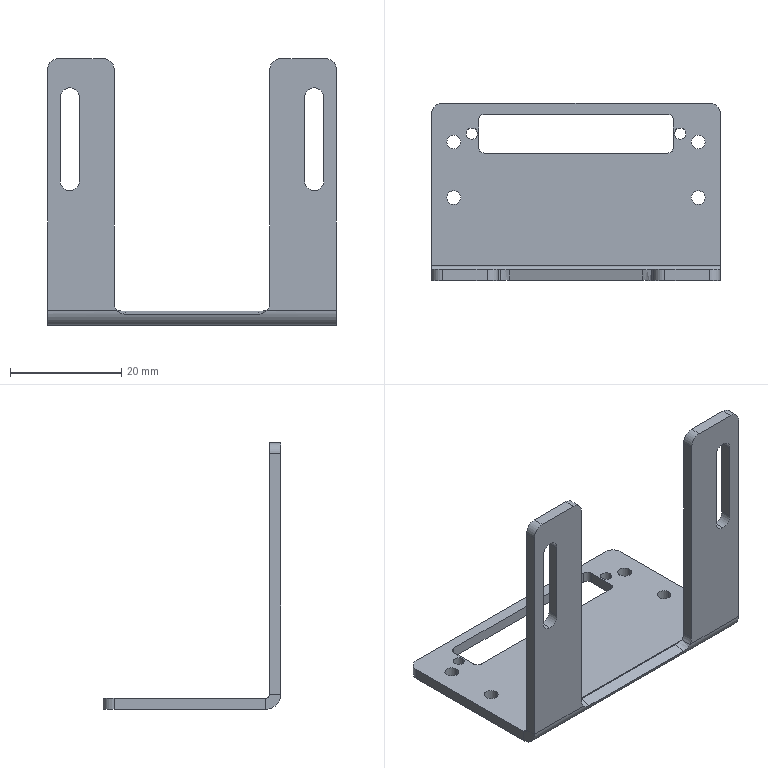Part | STEP file | 06-08 light source mounting plate A (Default) | 1 solid | 60 faces | box 52 x 32 x 48 mm | volume 4676 mm3 | cylinder 32 | plane 26 | spline 2 | commonest cylinder face diameters 2.5 x8 4 x8 3.5 x6 2 x4 2.05 x4 1.473 x1